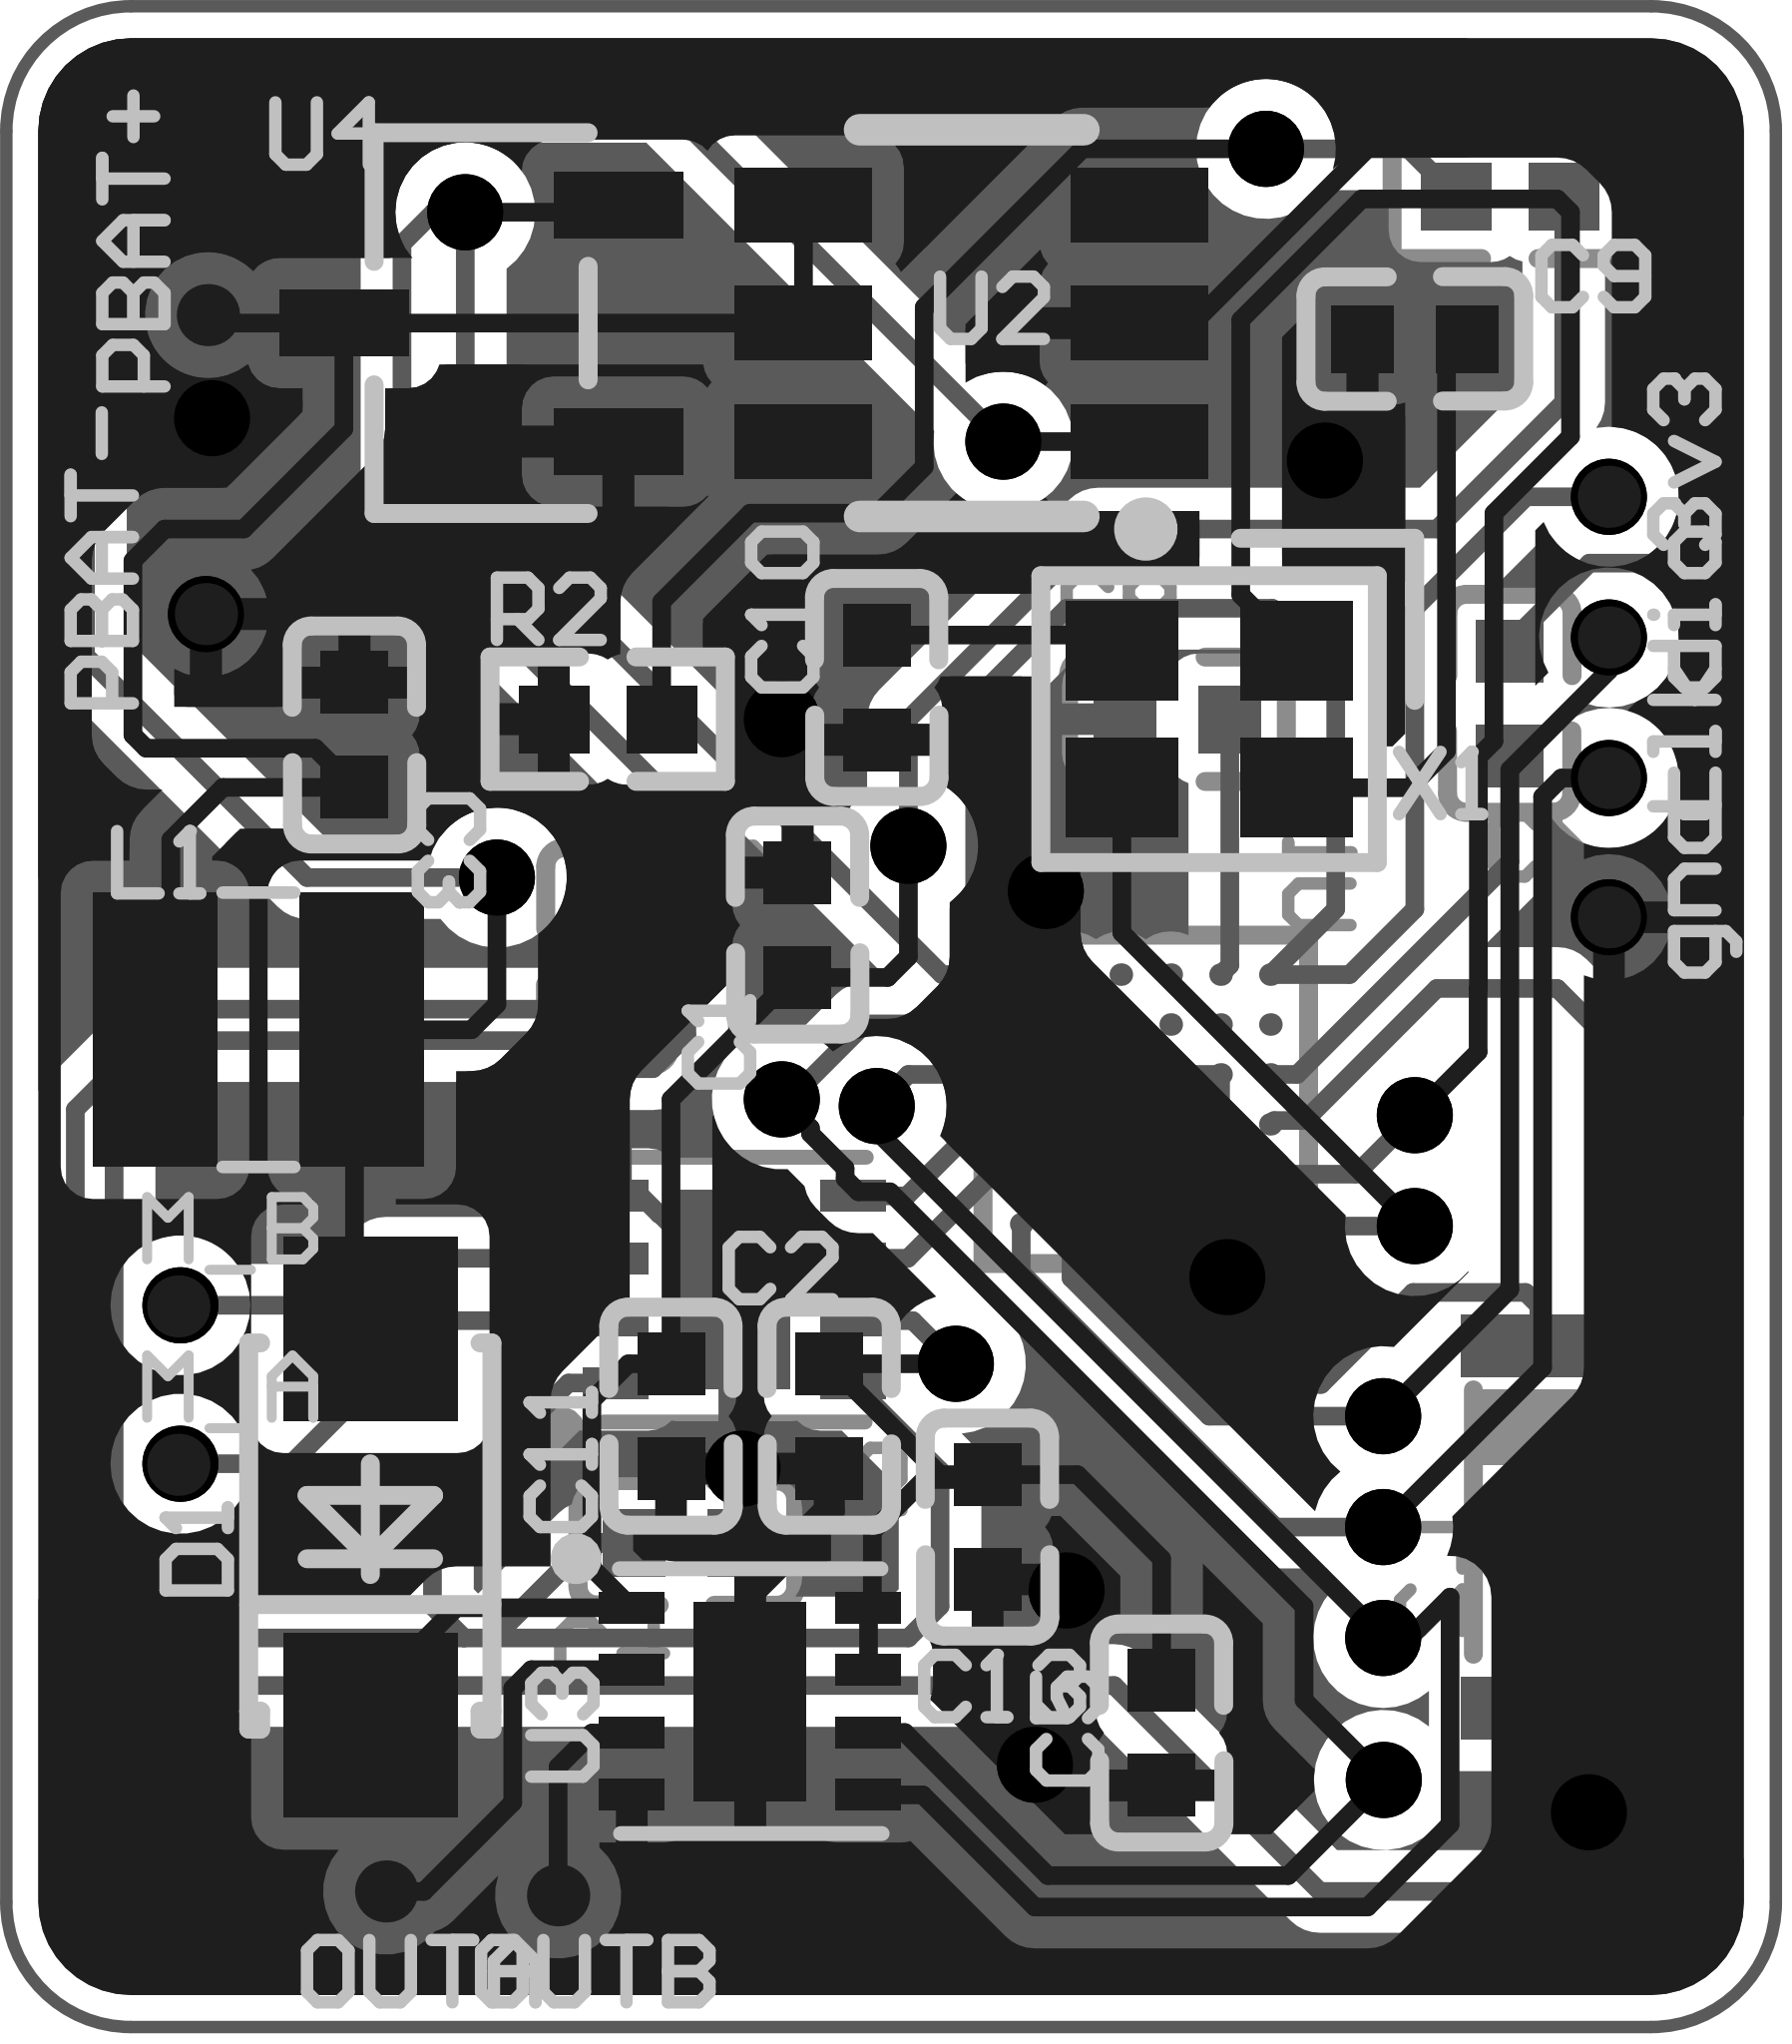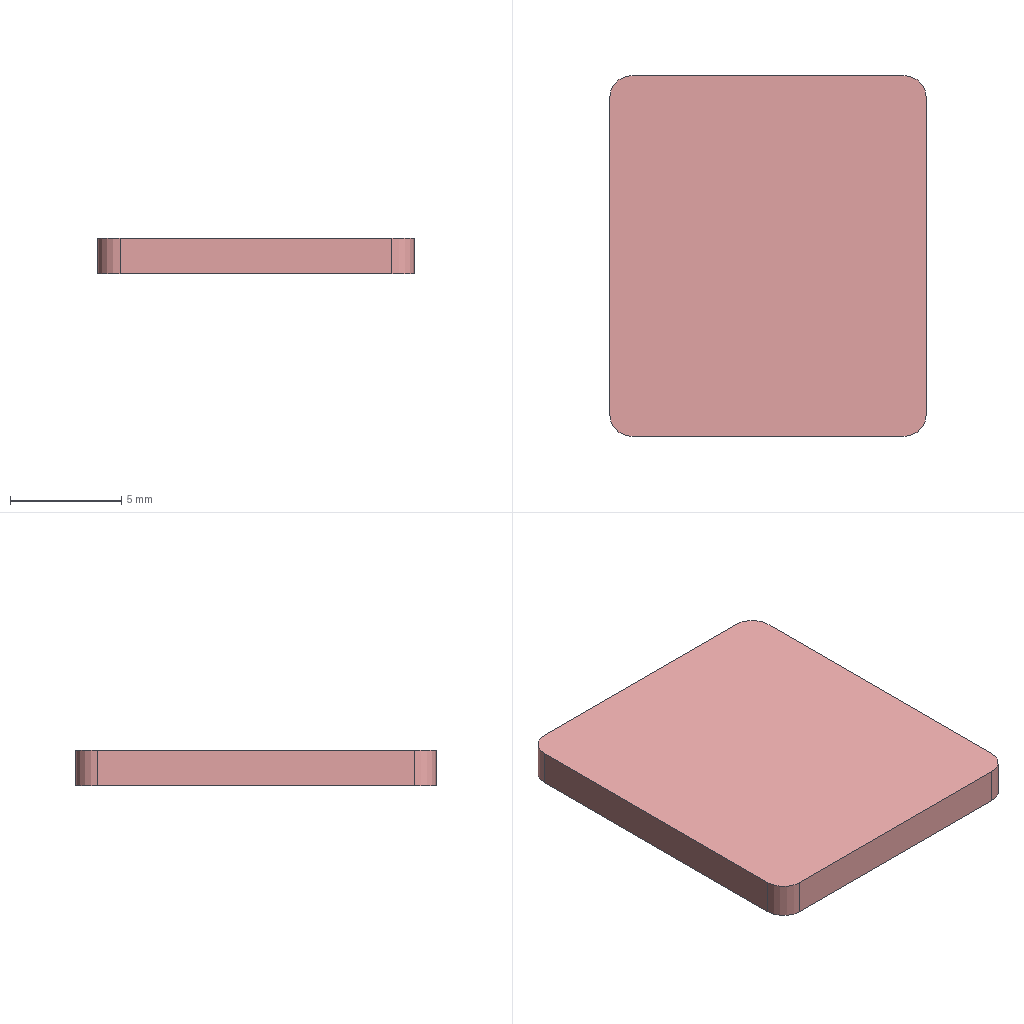Circuit board layout | Altium Designer | box 14.2 x 16.2 x 1.6 mm
Layer stack:
# Altium Designer layer stack of  (unit mm; dielectric type: 0 none, 1 core, 2 prepreg, 3 surface material)
index,name,kind,layer,copper_thickness_mm,dielectric_type,dielectric_thickness_mm,dielectric_material,dielectric_constant
0,Top Paste Mask Layer,other,,,,,,
1,Top Silkscreen Layer,other,,,,,,
2,Top Solder Mask Layer,dielectric,,,3,0.01,,3.3
3,Top Layer,copper,Top Layer,0.035,,,,
4,Dielectric1,dielectric,,,3,1.51,FR4,4.5
5,Bottom Layer,copper,Bottom Layer,0.035,,,,
6,Bottom Solder Mask Layer,dielectric,,,3,0.01,,3.3
7,Bottom Silkscreen Layer,other,,,,,,
8,Bottom Paste Mask Layer,other,,,,,,
# drill layer pairs: low layer,high layer
drill_pair,Top Layer,Bottom Layer
Part placement:
Designator,Comment,Layer,Footprint,Center-X(mm),Center-Y(mm),Rotation
C1,100nF,TopLayer,C0402,86.741,88.519,270
C2,100nF,TopLayer,C0402,86.995,84.582,90
C3,10uF,TopLayer,C0402,83.185,90.043,270
C4,10uF,BottomLayer,C0402,85.852,83.566,0
C6,100nF,BottomLayer,C0402,85.217,88.265,270
C7,100nF,BottomLayer,C0402,92.456,90.297,270
C8,100nF,BottomLayer,C0402,89.789,90.17,0
C9,12pF,TopLayer,C0402,91.694,93.218,0
C10,12pF,TopLayer,C0402,87.376,90.424,90
C11,100nF,TopLayer,C0402,85.725,84.582,90
D1,SS24L,TopLayer,SOD-123FL_L2.8-W1.8-LS3.7-R-RD,83.312,83.693,90
L1,4.7uH,TopLayer,IND-SMD_L2.5-W2.0_VLS2520X,82.414,87.68,180
L2,KH-3216-H0209,BottomLayer,ANT-SMD_L3.2-W1.6-KH-3216F245C04,92.964,83.693,270
3v3,,TopLayer,Test-Point-0.5mm,93.251,91.953,0
PBAT+,,TopLayer,Test-Point-0.5mm,82.009,93.409,0
PBAT-,,TopLayer,Test-Point-0.5mm,81.993,91.012,0
gnd,,TopLayer,Test-Point-0.5mm,93.251,88.582,0
OUTA,,TopLayer,Test-Point-0.5mm,83.439,80.772,0
OUTB,,TopLayer,Test-Point-0.5mm,84.819,80.741,0
clk,,TopLayer,Test-Point-0.5mm,93.251,89.698,0
dio,,TopLayer,Test-Point-0.5mm,93.251,90.825,0
R2,9.1kΩ,TopLayer,R0402,85.217,90.17,0
R3,110kΩ,BottomLayer,R0402,92.456,94.361,0
U1,NRF52810-CAAA-R,BottomLayer,WLCSP-33_L2.5-W2.5-P0.40_NRF52810-CAAA-R,89.535,87.122,90
U2,MSY7208ABC,TopLayer,SOT-23-6_L2.9-W1.6-P0.95-LS2.8-BR,88.138,93.345,0
U3,DRV8837DSGR,TopLayer,WSON-8_L2.0-W2.0-P0.50-TL-EP,86.36,82.296,0
U4,XC6206P332MR,TopLayer,SOT-23-3_L3.0-W1.7-P0.95-LS2.9-BR,84.201,93.345,0
X1,32MHz,TopLayer,CRYSTAL-SMD_4P-L2.0-W1.6-BL,90.043,90.17,180
C5,100nF,TopLayer,C0402,89.662,82.042,90
C13,10uF,TopLayer,C0402,88.265,83.693,270
M_A,,TopLayer,Test-Point-0.5mm,81.771,84.192,0
M_B,,TopLayer,Test-Point-0.5mm,81.771,85.462,0
U5,DRV8837DSGR,BottomLayer,WSON-8_L2.0-W2.0-P0.50-TL-EP,86.233,85.598,0
Pad and via stacks:
# Altium Designer via and pad stacks of  (unit mm). Each distinct definition once, with the count of objects using it.
# via: kind,start_layer,end_layer,hole_mm,diameter_mm,mode(0 simple;1 top-mid-bottom;2 full stack),diameter_per_layer,count,example_net
# pad: kind,layer,hole_mm,hole_type(0 round;1 square;2 slot),plating,top_size,top_shape(1 round;2 rect;3 octagon;9 rounded rect),mid_size,bottom_size,mode,footprint,size_per_layer,count,example
pad,Top Layer,0,0,plated,0.5x0.54,2,0.5x0.54,0.5x0.54,0,C0402,,16,C1.2
pad,Top Layer,0,0,plated,1.48x1.4,2,1.48x1.4,1.48x1.4,0,SOD-123FL_L2.8-W1.8-LS3.7-R-RD,,2,D1.1
pad,Top Layer,0,0,plated,1x2.2,2,1x2.2,1x2.2,0,IND-SMD_L2.5-W2.0_VLS2520X,,2,L1.1
pad,Top Layer,0,0,plated,0.5x0.5,1,0.5x0.5,0.5x0.5,0,Test-Point-0.5mm,,10,3v3.1
pad,Top Layer,0,0,plated,0.5657x0.54,2,0.5657x0.54,0.5657x0.54,0,R0402,,2,R2.2
pad,Top Layer,0,0,plated,1.1x0.6,2,1.1x0.6,1.1x0.6,0,SOT-23-6_L2.9-W1.6-P0.95-LS2.8-BR,,6,U2.3
pad,Top Layer,0,0,plated,0.521x0.25,2,0.521x0.25,0.521x0.25,0,WSON-8_L2.0-W2.0-P0.50-TL-EP,,8,U3.1
pad,Top Layer,0,0,plated,0.9x1.6,2,0.9x1.6,0.9x1.6,0,WSON-8_L2.0-W2.0-P0.50-TL-EP,,1,U3.9
pad,Top Layer,0,0,plated,1.038x0.532,2,1.038x0.532,1.038x0.532,0,SOT-23-3_L3.0-W1.7-P0.95-LS2.9-BR,,3,U4.1
pad,Top Layer,0,0,plated,0.9x0.8,2,0.9x0.8,0.9x0.8,0,CRYSTAL-SMD_4P-L2.0-W1.6-BL,,4,X1.2
pad,Bottom Layer,0,0,plated,0.5x0.54,2,0.5x0.54,0.5x0.54,0,C0402,,8,C4.2
pad,Bottom Layer,0,0,plated,0.5x1.8,2,0.5x1.8,0.5x1.8,0,ANT-SMD_L3.2-W1.6-KH-3216F245C04,,2,L2.1
pad,Bottom Layer,0,0,plated,0.5657x0.54,2,0.5657x0.54,0.5657x0.54,0,R0402,,2,R3.2
pad,Bottom Layer,0,0,plated,0.1816x0.1816,1,0.1816x0.1816,0.1816x0.1816,0,WLCSP-33_L2.5-W2.5-P0.40_NRF52810-CAAA-R,,33,U1.A1
pad,Bottom Layer,0,0,plated,0.521x0.25,2,0.521x0.25,0.521x0.25,0,WSON-8_L2.0-W2.0-P0.50-TL-EP,,8,U5.1
pad,Bottom Layer,0,0,plated,0.9x1.6,2,0.9x1.6,0.9x1.6,0,WSON-8_L2.0-W2.0-P0.50-TL-EP,,1,U5.9
via,Top Layer,Bottom Layer,0.3048,0.61,0,,30,3V3
Copper pours:
name,layer,net,type(0 solid;1 hatched;2 none)
Top Layer-GND,Top Layer,GND,0
Top Layer-GND 1,Top Layer,GND,0
Bottom Layer-GND,Bottom Layer,GND,0